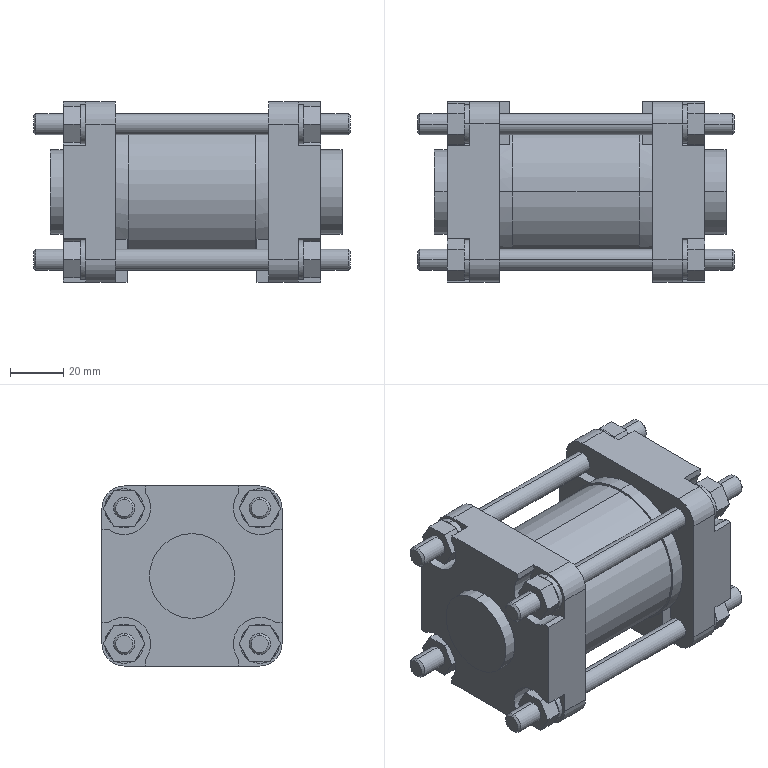Part | SolidWorks | features BaseBody 1 | 1 solid | 328 faces | box 119.6 x 68 x 68 mm | volume 285517 mm3 | plane 222 | cylinder 82 | cone 24 | commonest cylinder face diameters 8 x24 14.72 x16 20 x12 16.8 x8 7.84 x4 11.96 x4